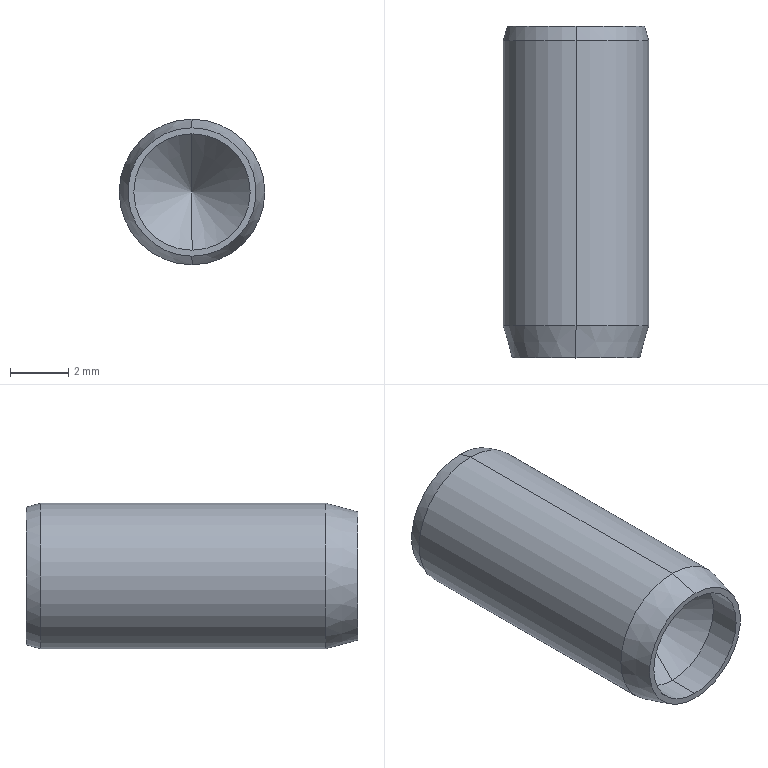Part | STEP file | 1 solid | 25 faces | box 5 x 11.4 x 5 mm | volume 186.144 mm3 | cone 10 | plane 9 | cylinder 6 | commonest cylinder face diameters 1.95 x2 4 x2 5 x2
STEP:
#1=CARTESIAN_POINT('',(0.,7.9,-0.975));
#2=VERTEX_POINT('',#1);
#3=CARTESIAN_POINT('',(0.,8.4,-0.975));
#4=VERTEX_POINT('',#3);
#5=CARTESIAN_POINT('',(0.,11.4,-0.975));
#6=DIRECTION('',(0.,1.,0.));
#7=VECTOR('',#6,1000.);
#8=LINE('',#5,#7);
#9=EDGE_CURVE('',#2,#4,#8,.T.);
#10=ORIENTED_EDGE('',*,*,#9,.F.);
#11=CARTESIAN_POINT('',(0.,7.9,0.975));
#12=VERTEX_POINT('',#11);
#13=CARTESIAN_POINT('',(0.,7.9,0.));
#14=DIRECTION('',(0.,1.,0.));
#15=DIRECTION('',(0.,0.,1.));
#16=AXIS2_PLACEMENT_3D('',#13,#14,#15);
#17=CIRCLE('',#16,0.975);
#18=EDGE_CURVE('',#12,#2,#17,.T.);
#19=ORIENTED_EDGE('',*,*,#18,.F.);
#20=CARTESIAN_POINT('',(0.,8.4,0.975));
#21=VERTEX_POINT('',#20);
#22=CARTESIAN_POINT('',(0.,11.4,0.975));
#23=DIRECTION('',(0.,1.,0.));
#24=VECTOR('',#23,1000.);
#25=LINE('',#22,#24);
#26=EDGE_CURVE('',#12,#21,#25,.T.);
#27=ORIENTED_EDGE('',*,*,#26,.T.);
#28=CARTESIAN_POINT('',(0.,8.4,0.));
#29=DIRECTION('',(0.,-1.,0.));
#30=DIRECTION('',(0.,0.,1.));
#31=AXIS2_PLACEMENT_3D('',#28,#29,#30);
#32=CIRCLE('',#31,0.975);
#33=EDGE_CURVE('',#4,#21,#32,.T.);
#34=ORIENTED_EDGE('',*,*,#33,.F.);
#35=EDGE_LOOP('',(#10,#19,#27,#34));
#36=FACE_OUTER_BOUND('',#35,.T.);
#37=CARTESIAN_POINT('',(0.,11.4,0.));
#38=DIRECTION('',(0.,1.,0.));
#39=DIRECTION('',(0.,0.,1.));
#40=AXIS2_PLACEMENT_3D('',#37,#38,#39);
#41=CYLINDRICAL_SURFACE('',#40,0.975);
#42=ADVANCED_FACE('',(#36),#41,.F.);
#43=CARTESIAN_POINT('',(0.,7.314,0.));
#44=VERTEX_POINT('',#43);
#45=CARTESIAN_POINT('',(0.,7.9,-0.975));
#46=DIRECTION('',(0.,0.515,-0.8572));
#47=VECTOR('',#46,1000.);
#48=LINE('',#45,#47);
#49=EDGE_CURVE('',#44,#2,#48,.T.);
#50=ORIENTED_EDGE('',*,*,#49,.F.);
#51=CARTESIAN_POINT('',(0.,7.9,0.975));
#52=DIRECTION('',(0.,0.515,0.8572));
#53=VECTOR('',#52,1000.);
#54=LINE('',#51,#53);
#55=EDGE_CURVE('',#44,#12,#54,.T.);
#56=ORIENTED_EDGE('',*,*,#55,.T.);
#57=ORIENTED_EDGE('',*,*,#18,.T.);
#58=EDGE_LOOP('',(#50,#56,#57));
#59=FACE_OUTER_BOUND('',#58,.T.);
#60=CARTESIAN_POINT('',(0.,7.9,0.));
#61=DIRECTION('',(0.,1.,0.));
#62=DIRECTION('',(0.,0.,1.));
#63=AXIS2_PLACEMENT_3D('',#60,#61,#62);
#64=CONICAL_SURFACE('',#63,0.975,1.03);
#65=ADVANCED_FACE('',(#59),#64,.F.);
#66=CARTESIAN_POINT('',(1.155,11.38,0.));
#67=VERTEX_POINT('',#66);
#68=CARTESIAN_POINT('',(0.5774,11.38,-1.));
#69=VERTEX_POINT('',#68);
#70=CARTESIAN_POINT('',(1.155,11.38,0.));
#71=CARTESIAN_POINT('',(1.104,11.329,-0.08728));
#72=CARTESIAN_POINT('',(1.031,11.272,-0.215));
#73=CARTESIAN_POINT('',(0.9596,11.243,-0.338));
#74=CARTESIAN_POINT('',(0.9129,11.229,-0.4189));
#75=CARTESIAN_POINT('',(0.889,11.226,-0.4602));
#76=CARTESIAN_POINT('',(0.7793,11.223,-0.6502));
#77=CARTESIAN_POINT('',(0.6828,11.274,-0.8174));
#78=CARTESIAN_POINT('',(0.5774,11.38,-1.));
#79=B_SPLINE_CURVE_WITH_KNOTS('',3,(#70,#71,#72,#73,#74,#75,#76,#77,#78),.UNSPECIFIED.,.F.,.F.,(4,1,2,2,4),(0.,0.25,0.375,0.5,1.),.UNSPECIFIED.);
#80=EDGE_CURVE('',#67,#69,#79,.T.);
#81=ORIENTED_EDGE('',*,*,#80,.T.);
#82=CARTESIAN_POINT('',(0.5774,8.4,-1.));
#83=VERTEX_POINT('',#82);
#84=CARTESIAN_POINT('',(0.5774,8.4,-1.));
#85=DIRECTION('',(0.,1.,0.));
#86=VECTOR('',#85,1000.);
#87=LINE('',#84,#86);
#88=EDGE_CURVE('',#83,#69,#87,.T.);
#89=ORIENTED_EDGE('',*,*,#88,.F.);
#90=CARTESIAN_POINT('',(1.155,8.4,0.));
#91=VERTEX_POINT('',#90);
#92=CARTESIAN_POINT('',(1.155,8.4,0.));
#93=DIRECTION('',(-0.5,0.,-0.866));
#94=VECTOR('',#93,1000.);
#95=LINE('',#92,#94);
#96=EDGE_CURVE('',#91,#83,#95,.T.);
#97=ORIENTED_EDGE('',*,*,#96,.F.);
#98=CARTESIAN_POINT('',(1.155,8.4,0.));
#99=DIRECTION('',(0.,1.,0.));
#100=VECTOR('',#99,1000.);
#101=LINE('',#98,#100);
#102=EDGE_CURVE('',#91,#67,#101,.T.);
#103=ORIENTED_EDGE('',*,*,#102,.T.);
#104=EDGE_LOOP('',(#81,#89,#97,#103));
#105=FACE_OUTER_BOUND('',#104,.T.);
#106=CARTESIAN_POINT('',(1.155,8.4,0.));
#107=DIRECTION('',(0.866,0.,-0.5));
#108=DIRECTION('',(0.,-1.,0.));
#109=AXIS2_PLACEMENT_3D('',#106,#107,#108);
#110=PLANE('',#109);
#111=ADVANCED_FACE('',(#105),#110,.F.);
#112=CARTESIAN_POINT('',(0.,11.225,-1.));
#113=VERTEX_POINT('',#112);
#114=CARTESIAN_POINT('',(0.5774,11.38,-1.));
#115=CARTESIAN_POINT('',(0.3711,11.277,-1.));
#116=CARTESIAN_POINT('',(0.1786,11.225,-1.));
#117=CARTESIAN_POINT('',(0.,11.225,-1.));
#118=B_SPLINE_CURVE_WITH_KNOTS('',3,(#114,#115,#116,#117),.UNSPECIFIED.,.F.,.F.,(4,4),(0.,1.),.UNSPECIFIED.);
#119=EDGE_CURVE('',#69,#113,#118,.T.);
#120=ORIENTED_EDGE('',*,*,#119,.T.);
#121=CARTESIAN_POINT('',(-0.5774,11.38,-1.));
#122=VERTEX_POINT('',#121);
#123=CARTESIAN_POINT('',(0.,11.225,-1.));
#124=CARTESIAN_POINT('',(-0.1786,11.225,-1.));
#125=CARTESIAN_POINT('',(-0.3711,11.277,-1.));
#126=CARTESIAN_POINT('',(-0.5774,11.38,-1.));
#127=B_SPLINE_CURVE_WITH_KNOTS('',3,(#123,#124,#125,#126),.UNSPECIFIED.,.F.,.F.,(4,4),(0.,1.),.UNSPECIFIED.);
#128=EDGE_CURVE('',#113,#122,#127,.T.);
#129=ORIENTED_EDGE('',*,*,#128,.T.);
#130=CARTESIAN_POINT('',(-0.5774,8.4,-1.));
#131=VERTEX_POINT('',#130);
#132=CARTESIAN_POINT('',(-0.5774,8.4,-1.));
#133=DIRECTION('',(0.,1.,0.));
#134=VECTOR('',#133,1000.);
#135=LINE('',#132,#134);
#136=EDGE_CURVE('',#131,#122,#135,.T.);
#137=ORIENTED_EDGE('',*,*,#136,.F.);
#138=CARTESIAN_POINT('',(0.5774,8.4,-1.));
#139=DIRECTION('',(-1.,0.,0.));
#140=VECTOR('',#139,1000.);
#141=LINE('',#138,#140);
#142=EDGE_CURVE('',#83,#131,#141,.T.);
#143=ORIENTED_EDGE('',*,*,#142,.F.);
#144=ORIENTED_EDGE('',*,*,#88,.T.);
#145=EDGE_LOOP('',(#120,#129,#137,#143,#144));
#146=FACE_OUTER_BOUND('',#145,.T.);
#147=CARTESIAN_POINT('',(0.5774,8.4,-1.));
#148=DIRECTION('',(0.,0.,-1.));
#149=DIRECTION('',(0.,-1.,0.));
#150=AXIS2_PLACEMENT_3D('',#147,#148,#149);
#151=PLANE('',#150);
#152=ADVANCED_FACE('',(#146),#151,.F.);
#153=CARTESIAN_POINT('',(-1.155,11.38,0.));
#154=VERTEX_POINT('',#153);
#155=CARTESIAN_POINT('',(-0.5774,11.38,-1.));
#156=CARTESIAN_POINT('',(-0.6277,11.329,-0.9127));
#157=CARTESIAN_POINT('',(-0.7015,11.272,-0.785));
#158=CARTESIAN_POINT('',(-0.7725,11.243,-0.662));
#159=CARTESIAN_POINT('',(-0.8192,11.229,-0.5811));
#160=CARTESIAN_POINT('',(-0.843,11.226,-0.5398));
#161=CARTESIAN_POINT('',(-0.9527,11.223,-0.3498));
#162=CARTESIAN_POINT('',(-1.049,11.274,-0.1826));
#163=CARTESIAN_POINT('',(-1.155,11.38,0.));
#164=B_SPLINE_CURVE_WITH_KNOTS('',3,(#155,#156,#157,#158,#159,#160,#161,#162,#163),.UNSPECIFIED.,.F.,.F.,(4,1,2,2,4),(0.,0.25,0.375,0.5,1.),.UNSPECIFIED.);
#165=EDGE_CURVE('',#122,#154,#164,.T.);
#166=ORIENTED_EDGE('',*,*,#165,.T.);
#167=CARTESIAN_POINT('',(-1.155,8.4,0.));
#168=VERTEX_POINT('',#167);
#169=CARTESIAN_POINT('',(-1.155,8.4,0.));
#170=DIRECTION('',(0.,1.,0.));
#171=VECTOR('',#170,1000.);
#172=LINE('',#169,#171);
#173=EDGE_CURVE('',#168,#154,#172,.T.);
#174=ORIENTED_EDGE('',*,*,#173,.F.);
#175=CARTESIAN_POINT('',(-0.5774,8.4,-1.));
#176=DIRECTION('',(-0.5,0.,0.866));
#177=VECTOR('',#176,1000.);
#178=LINE('',#175,#177);
#179=EDGE_CURVE('',#131,#168,#178,.T.);
#180=ORIENTED_EDGE('',*,*,#179,.F.);
#181=ORIENTED_EDGE('',*,*,#136,.T.);
#182=EDGE_LOOP('',(#166,#174,#180,#181));
#183=FACE_OUTER_BOUND('',#182,.T.);
#184=CARTESIAN_POINT('',(-0.5774,8.4,-1.));
#185=DIRECTION('',(-0.866,0.,-0.5));
#186=DIRECTION('',(-0.5,0.,0.866));
#187=AXIS2_PLACEMENT_3D('',#184,#185,#186);
#188=PLANE('',#187);
#189=ADVANCED_FACE('',(#183),#188,.F.);
#190=CARTESIAN_POINT('',(-0.5774,11.38,1.));
#191=VERTEX_POINT('',#190);
#192=CARTESIAN_POINT('',(-1.155,11.38,0.));
#193=CARTESIAN_POINT('',(-1.104,11.329,0.08728));
#194=CARTESIAN_POINT('',(-1.031,11.272,0.215));
#195=CARTESIAN_POINT('',(-0.9596,11.243,0.338));
#196=CARTESIAN_POINT('',(-0.9129,11.229,0.4189));
#197=CARTESIAN_POINT('',(-0.889,11.226,0.4602));
#198=CARTESIAN_POINT('',(-0.7793,11.223,0.6502));
#199=CARTESIAN_POINT('',(-0.6828,11.274,0.8174));
#200=CARTESIAN_POINT('',(-0.5774,11.38,1.));
#201=B_SPLINE_CURVE_WITH_KNOTS('',3,(#192,#193,#194,#195,#196,#197,#198,#199,#200),.UNSPECIFIED.,.F.,.F.,(4,1,2,2,4),(0.,0.25,0.375,0.5,1.),.UNSPECIFIED.);
#202=EDGE_CURVE('',#154,#191,#201,.T.);
#203=ORIENTED_EDGE('',*,*,#202,.T.);
#204=CARTESIAN_POINT('',(-0.5774,8.4,1.));
#205=VERTEX_POINT('',#204);
#206=CARTESIAN_POINT('',(-0.5774,8.4,1.));
#207=DIRECTION('',(0.,1.,0.));
#208=VECTOR('',#207,1000.);
#209=LINE('',#206,#208);
#210=EDGE_CURVE('',#205,#191,#209,.T.);
#211=ORIENTED_EDGE('',*,*,#210,.F.);
#212=CARTESIAN_POINT('',(-1.155,8.4,0.));
#213=DIRECTION('',(0.5,0.,0.866));
#214=VECTOR('',#213,1000.);
#215=LINE('',#212,#214);
#216=EDGE_CURVE('',#168,#205,#215,.T.);
#217=ORIENTED_EDGE('',*,*,#216,.F.);
#218=ORIENTED_EDGE('',*,*,#173,.T.);
#219=EDGE_LOOP('',(#203,#211,#217,#218));
#220=FACE_OUTER_BOUND('',#219,.T.);
#221=CARTESIAN_POINT('',(-1.155,8.4,0.));
#222=DIRECTION('',(-0.866,0.,0.5));
#223=DIRECTION('',(0.,1.,0.));
#224=AXIS2_PLACEMENT_3D('',#221,#222,#223);
#225=PLANE('',#224);
#226=ADVANCED_FACE('',(#220),#225,.F.);
#227=CARTESIAN_POINT('',(0.,11.225,1.));
#228=VERTEX_POINT('',#227);
#229=CARTESIAN_POINT('',(-0.5774,11.38,1.));
#230=CARTESIAN_POINT('',(-0.3711,11.277,1.));
#231=CARTESIAN_POINT('',(-0.1786,11.225,1.));
#232=CARTESIAN_POINT('',(0.,11.225,1.));
#233=B_SPLINE_CURVE_WITH_KNOTS('',3,(#229,#230,#231,#232),.UNSPECIFIED.,.F.,.F.,(4,4),(0.,1.),.UNSPECIFIED.);
#234=EDGE_CURVE('',#191,#228,#233,.T.);
#235=ORIENTED_EDGE('',*,*,#234,.T.);
#236=CARTESIAN_POINT('',(0.5774,11.38,1.));
#237=VERTEX_POINT('',#236);
#238=CARTESIAN_POINT('',(0.,11.225,1.));
#239=CARTESIAN_POINT('',(0.1786,11.225,1.));
#240=CARTESIAN_POINT('',(0.3711,11.277,1.));
#241=CARTESIAN_POINT('',(0.5774,11.38,1.));
#242=B_SPLINE_CURVE_WITH_KNOTS('',3,(#238,#239,#240,#241),.UNSPECIFIED.,.F.,.F.,(4,4),(0.,1.),.UNSPECIFIED.);
#243=EDGE_CURVE('',#228,#237,#242,.T.);
#244=ORIENTED_EDGE('',*,*,#243,.T.);
#245=CARTESIAN_POINT('',(0.5774,8.4,1.));
#246=VERTEX_POINT('',#245);
#247=CARTESIAN_POINT('',(0.5774,8.4,1.));
#248=DIRECTION('',(0.,1.,0.));
#249=VECTOR('',#248,1000.);
#250=LINE('',#247,#249);
#251=EDGE_CURVE('',#246,#237,#250,.T.);
#252=ORIENTED_EDGE('',*,*,#251,.F.);
#253=CARTESIAN_POINT('',(-0.5774,8.4,1.));
#254=DIRECTION('',(1.,0.,0.));
#255=VECTOR('',#254,1000.);
#256=LINE('',#253,#255);
#257=EDGE_CURVE('',#205,#246,#256,.T.);
#258=ORIENTED_EDGE('',*,*,#257,.F.);
#259=ORIENTED_EDGE('',*,*,#210,.T.);
#260=EDGE_LOOP('',(#235,#244,#252,#258,#259));
#261=FACE_OUTER_BOUND('',#260,.T.);
#262=CARTESIAN_POINT('',(-0.5774,8.4,1.));
#263=DIRECTION('',(0.,0.,1.));
#264=DIRECTION('',(0.,-1.,0.));
#265=AXIS2_PLACEMENT_3D('',#262,#263,#264);
#266=PLANE('',#265);
#267=ADVANCED_FACE('',(#261),#266,.F.);
#268=CARTESIAN_POINT('',(0.5774,11.38,1.));
#269=CARTESIAN_POINT('',(0.6277,11.329,0.9127));
#270=CARTESIAN_POINT('',(0.7015,11.272,0.785));
#271=CARTESIAN_POINT('',(0.7725,11.243,0.662));
#272=CARTESIAN_POINT('',(0.8192,11.229,0.5811));
#273=CARTESIAN_POINT('',(0.843,11.226,0.5398));
#274=CARTESIAN_POINT('',(0.9527,11.223,0.3498));
#275=CARTESIAN_POINT('',(1.049,11.274,0.1826));
#276=CARTESIAN_POINT('',(1.155,11.38,0.));
#277=B_SPLINE_CURVE_WITH_KNOTS('',3,(#268,#269,#270,#271,#272,#273,#274,#275,#276),.UNSPECIFIED.,.F.,.F.,(4,1,2,2,4),(0.,0.25,0.375,0.5,1.),.UNSPECIFIED.);
#278=EDGE_CURVE('',#237,#67,#277,.T.);
#279=ORIENTED_EDGE('',*,*,#278,.T.);
#280=ORIENTED_EDGE('',*,*,#102,.F.);
#281=CARTESIAN_POINT('',(0.5774,8.4,1.));
#282=DIRECTION('',(0.5,0.,-0.866));
#283=VECTOR('',#282,1000.);
#284=LINE('',#281,#283);
#285=EDGE_CURVE('',#246,#91,#284,.T.);
#286=ORIENTED_EDGE('',*,*,#285,.F.);
#287=ORIENTED_EDGE('',*,*,#251,.T.);
#288=EDGE_LOOP('',(#279,#280,#286,#287));
#289=FACE_OUTER_BOUND('',#288,.T.);
#290=CARTESIAN_POINT('',(0.5774,8.4,1.));
#291=DIRECTION('',(0.866,0.,0.5));
#292=DIRECTION('',(0.,-1.,0.));
#293=AXIS2_PLACEMENT_3D('',#290,#291,#292);
#294=PLANE('',#293);
#295=ADVANCED_FACE('',(#289),#294,.F.);
#296=CARTESIAN_POINT('',(0.,8.4,0.));
#297=DIRECTION('',(0.,-1.,0.));
#298=DIRECTION('',(0.,0.,1.));
#299=AXIS2_PLACEMENT_3D('',#296,#297,#298);
#300=CIRCLE('',#299,0.975);
#301=EDGE_CURVE('',#21,#4,#300,.T.);
#302=ORIENTED_EDGE('',*,*,#301,.T.);
#303=ORIENTED_EDGE('',*,*,#33,.T.);
#304=EDGE_LOOP('',(#302,#303));
#305=FACE_BOUND('',#304,.T.);
#306=ORIENTED_EDGE('',*,*,#285,.T.);
#307=ORIENTED_EDGE('',*,*,#96,.T.);
#308=ORIENTED_EDGE('',*,*,#142,.T.);
#309=ORIENTED_EDGE('',*,*,#179,.T.);
#310=ORIENTED_EDGE('',*,*,#216,.T.);
#311=ORIENTED_EDGE('',*,*,#257,.T.);
#312=EDGE_LOOP('',(#306,#307,#308,#309,#310,#311));
#313=FACE_OUTER_BOUND('',#312,.T.);
#314=CARTESIAN_POINT('',(0.,8.4,0.));
#315=DIRECTION('',(0.,1.,0.));
#316=DIRECTION('',(1.,0.,0.));
#317=AXIS2_PLACEMENT_3D('',#314,#315,#316);
#318=PLANE('',#317);
#319=ADVANCED_FACE('',(#305,#313),#318,.T.);
#320=CARTESIAN_POINT('',(0.,11.4,-1.175));
#321=VERTEX_POINT('',#320);
#322=CARTESIAN_POINT('',(0.,11.2,-0.975));
#323=DIRECTION('',(0.,0.7071,-0.7071));
#324=VECTOR('',#323,1000.);
#325=LINE('',#322,#324);
#326=EDGE_CURVE('',#113,#321,#325,.T.);
#327=ORIENTED_EDGE('',*,*,#326,.F.);
#328=ORIENTED_EDGE('',*,*,#119,.F.);
#329=ORIENTED_EDGE('',*,*,#80,.F.);
#330=ORIENTED_EDGE('',*,*,#278,.F.);
#331=ORIENTED_EDGE('',*,*,#243,.F.);
#332=CARTESIAN_POINT('',(0.,11.4,1.175));
#333=VERTEX_POINT('',#332);
#334=CARTESIAN_POINT('',(0.,11.2,0.975));
#335=DIRECTION('',(0.,0.7071,0.7071));
#336=VECTOR('',#335,1000.);
#337=LINE('',#334,#336);
#338=EDGE_CURVE('',#228,#333,#337,.T.);
#339=ORIENTED_EDGE('',*,*,#338,.T.);
#340=CARTESIAN_POINT('',(0.,11.4,0.));
#341=DIRECTION('',(0.,-1.,0.));
#342=DIRECTION('',(0.,0.,1.));
#343=AXIS2_PLACEMENT_3D('',#340,#341,#342);
#344=CIRCLE('',#343,1.175);
#345=EDGE_CURVE('',#321,#333,#344,.T.);
#346=ORIENTED_EDGE('',*,*,#345,.F.);
#347=EDGE_LOOP('',(#327,#328,#329,#330,#331,#339,#346));
#348=FACE_OUTER_BOUND('',#347,.T.);
#349=CARTESIAN_POINT('',(0.,11.2,0.));
#350=DIRECTION('',(0.,1.,0.));
#351=DIRECTION('',(0.,0.,1.));
#352=AXIS2_PLACEMENT_3D('',#349,#350,#351);
#353=CONICAL_SURFACE('',#352,0.975,0.7854);
#354=ADVANCED_FACE('',(#348),#353,.F.);
#355=CARTESIAN_POINT('',(0.,3.1,0.));
#356=VERTEX_POINT('',#355);
#357=CARTESIAN_POINT('',(0.,1.1,2.));
#358=VERTEX_POINT('',#357);
#359=CARTESIAN_POINT('',(0.,3.1,0.));
#360=DIRECTION('',(0.,-0.7071,0.7071));
#361=VECTOR('',#360,1000.);
#362=LINE('',#359,#361);
#363=EDGE_CURVE('',#356,#358,#362,.T.);
#364=ORIENTED_EDGE('',*,*,#363,.F.);
#365=CARTESIAN_POINT('',(0.,1.1,-2.));
#366=VERTEX_POINT('',#365);
#367=CARTESIAN_POINT('',(0.,3.1,0.));
#368=DIRECTION('',(0.,-0.7071,-0.7071));
#369=VECTOR('',#368,1000.);
#370=LINE('',#367,#369);
#371=EDGE_CURVE('',#356,#366,#370,.T.);
#372=ORIENTED_EDGE('',*,*,#371,.T.);
#373=CARTESIAN_POINT('',(0.,1.1,0.));
#374=DIRECTION('',(0.,-1.,0.));
#375=DIRECTION('',(0.,0.,-1.));
#376=AXIS2_PLACEMENT_3D('',#373,#374,#375);
#377=CIRCLE('',#376,2.);
#378=EDGE_CURVE('',#366,#358,#377,.T.);
#379=ORIENTED_EDGE('',*,*,#378,.T.);
#380=EDGE_LOOP('',(#364,#372,#379));
#381=FACE_OUTER_BOUND('',#380,.T.);
#382=CARTESIAN_POINT('',(0.,-996.9,0.));
#383=DIRECTION('',(0.,-1.,0.));
#384=DIRECTION('',(0.,0.,-1.));
#385=AXIS2_PLACEMENT_3D('',#382,#383,#384);
#386=CONICAL_SURFACE('',#385,1000.,0.7854);
#387=ADVANCED_FACE('',(#381),#386,.F.);
#388=CARTESIAN_POINT('',(0.,0.,2.));
#389=VERTEX_POINT('',#388);
#390=CARTESIAN_POINT('',(0.,0.,2.));
#391=DIRECTION('',(0.,-1.,0.));
#392=VECTOR('',#391,1000.);
#393=LINE('',#390,#392);
#394=EDGE_CURVE('',#358,#389,#393,.T.);
#395=ORIENTED_EDGE('',*,*,#394,.F.);
#396=ORIENTED_EDGE('',*,*,#378,.F.);
#397=CARTESIAN_POINT('',(0.,0.,-2.));
#398=VERTEX_POINT('',#397);
#399=CARTESIAN_POINT('',(0.,0.,-2.));
#400=DIRECTION('',(0.,-1.,0.));
#401=VECTOR('',#400,1000.);
#402=LINE('',#399,#401);
#403=EDGE_CURVE('',#366,#398,#402,.T.);
#404=ORIENTED_EDGE('',*,*,#403,.T.);
#405=CARTESIAN_POINT('',(0.,0.,0.));
#406=DIRECTION('',(0.,-1.,0.));
#407=DIRECTION('',(0.,0.,-1.));
#408=AXIS2_PLACEMENT_3D('',#405,#406,#407);
#409=CIRCLE('',#408,2.);
#410=EDGE_CURVE('',#398,#389,#409,.T.);
#411=ORIENTED_EDGE('',*,*,#410,.T.);
#412=EDGE_LOOP('',(#395,#396,#404,#411));
#413=FACE_OUTER_BOUND('',#412,.T.);
#414=CARTESIAN_POINT('',(0.,0.,0.));
#415=DIRECTION('',(0.,-1.,0.));
#416=DIRECTION('',(0.,0.,-1.));
#417=AXIS2_PLACEMENT_3D('',#414,#415,#416);
#418=CYLINDRICAL_SURFACE('',#417,2.);
#419=ADVANCED_FACE('',(#413),#418,.F.);
#420=CARTESIAN_POINT('',(0.,0.,-2.205));
#421=VERTEX_POINT('',#420);
#422=CARTESIAN_POINT('',(0.,1.1,-2.5));
#423=VERTEX_POINT('',#422);
#424=CARTESIAN_POINT('',(0.,1.1,-2.5));
#425=DIRECTION('',(0.,0.9659,-0.2588));
#426=VECTOR('',#425,1000.);
#427=LINE('',#424,#426);
#428=EDGE_CURVE('',#421,#423,#427,.T.);
#429=ORIENTED_EDGE('',*,*,#428,.F.);
#430=CARTESIAN_POINT('',(0.,0.,2.205));
#431=VERTEX_POINT('',#430);
#432=CARTESIAN_POINT('',(0.,0.,0.));
#433=DIRECTION('',(0.,-1.,0.));
#434=DIRECTION('',(0.,0.,1.));
#435=AXIS2_PLACEMENT_3D('',#432,#433,#434);
#436=CIRCLE('',#435,2.205);
#437=EDGE_CURVE('',#431,#421,#436,.T.);
#438=ORIENTED_EDGE('',*,*,#437,.F.);
#439=CARTESIAN_POINT('',(0.,1.1,2.5));
#440=VERTEX_POINT('',#439);
#441=CARTESIAN_POINT('',(0.,1.1,2.5));
#442=DIRECTION('',(0.,0.9659,0.2588));
#443=VECTOR('',#442,1000.);
#444=LINE('',#441,#443);
#445=EDGE_CURVE('',#431,#440,#444,.T.);
#446=ORIENTED_EDGE('',*,*,#445,.T.);
#447=CARTESIAN_POINT('',(0.,1.1,0.));
#448=DIRECTION('',(0.,1.,0.));
#449=DIRECTION('',(0.,0.,1.));
#450=AXIS2_PLACEMENT_3D('',#447,#448,#449);
#451=CIRCLE('',#450,2.5);
#452=EDGE_CURVE('',#423,#440,#451,.T.);
#453=ORIENTED_EDGE('',*,*,#452,.F.);
#454=EDGE_LOOP('',(#429,#438,#446,#453));
#455=FACE_OUTER_BOUND('',#454,.T.);
#456=CARTESIAN_POINT('',(0.,1.1,0.));
#457=DIRECTION('',(0.,1.,0.));
#458=DIRECTION('',(0.,0.,1.));
#459=AXIS2_PLACEMENT_3D('',#456,#457,#458);
#460=CONICAL_SURFACE('',#459,2.5,0.2618);
#461=ADVANCED_FACE('',(#455),#460,.T.);
#462=CARTESIAN_POINT('',(0.,11.4,2.366));
#463=VERTEX_POINT('',#462);
#464=CARTESIAN_POINT('',(0.,10.9,2.5));
#465=VERTEX_POINT('',#464);
#466=CARTESIAN_POINT('',(0.,11.4,2.366));
#467=DIRECTION('',(0.,-0.9659,0.2588));
#468=VECTOR('',#467,1000.);
#469=LINE('',#466,#468);
#470=EDGE_CURVE('',#463,#465,#469,.T.);
#471=ORIENTED_EDGE('',*,*,#470,.F.);
#472=CARTESIAN_POINT('',(0.,11.4,-2.366));
#473=VERTEX_POINT('',#472);
#474=CARTESIAN_POINT('',(0.,11.4,0.));
#475=DIRECTION('',(0.,1.,0.));
#476=DIRECTION('',(0.,0.,1.));
#477=AXIS2_PLACEMENT_3D('',#474,#475,#476);
#478=CIRCLE('',#477,2.366);
#479=EDGE_CURVE('',#473,#463,#478,.T.);
#480=ORIENTED_EDGE('',*,*,#479,.F.);
#481=CARTESIAN_POINT('',(0.,10.9,-2.5));
#482=VERTEX_POINT('',#481);
#483=CARTESIAN_POINT('',(0.,11.4,-2.366));
#484=DIRECTION('',(0.,-0.9659,-0.2588));
#485=VECTOR('',#484,1000.);
#486=LINE('',#483,#485);
#487=EDGE_CURVE('',#473,#482,#486,.T.);
#488=ORIENTED_EDGE('',*,*,#487,.T.);
#489=CARTESIAN_POINT('',(0.,10.9,0.));
#490=DIRECTION('',(0.,-1.,0.));
#491=DIRECTION('',(0.,0.,1.));
#492=AXIS2_PLACEMENT_3D('',#489,#490,#491);
#493=CIRCLE('',#492,2.5);
#494=EDGE_CURVE('',#465,#482,#493,.T.);
#495=ORIENTED_EDGE('',*,*,#494,.F.);
#496=EDGE_LOOP('',(#471,#480,#488,#495));
#497=FACE_OUTER_BOUND('',#496,.T.);
#498=CARTESIAN_POINT('',(0.,11.4,0.));
#499=DIRECTION('',(0.,-1.,0.));
#500=DIRECTION('',(0.,0.,-1.));
#501=AXIS2_PLACEMENT_3D('',#498,#499,#500);
#502=CONICAL_SURFACE('',#501,2.366,0.2618);
#503=ADVANCED_FACE('',(#497),#502,.T.);
#504=ORIENTED_EDGE('',*,*,#410,.F.);
#505=CARTESIAN_POINT('',(0.,0.,0.));
#506=DIRECTION('',(0.,-1.,0.));
#507=DIRECTION('',(0.,0.,-1.));
#508=AXIS2_PLACEMENT_3D('',#505,#506,#507);
#509=CIRCLE('',#508,2.);
#510=EDGE_CURVE('',#389,#398,#509,.T.);
#511=ORIENTED_EDGE('',*,*,#510,.F.);
#512=EDGE_LOOP('',(#504,#511));
#513=FACE_BOUND('',#512,.T.);
#514=ORIENTED_EDGE('',*,*,#437,.T.);
#515=CARTESIAN_POINT('',(0.,0.,0.));
#516=DIRECTION('',(0.,-1.,0.));
#517=DIRECTION('',(0.,0.,1.));
#518=AXIS2_PLACEMENT_3D('',#515,#516,#517);
#519=CIRCLE('',#518,2.205);
#520=EDGE_CURVE('',#421,#431,#519,.T.);
#521=ORIENTED_EDGE('',*,*,#520,.T.);
#522=EDGE_LOOP('',(#514,#521));
#523=FACE_OUTER_BOUND('',#522,.T.);
#524=CARTESIAN_POINT('',(0.,0.,0.));
#525=DIRECTION('',(0.,1.,0.));
#526=DIRECTION('',(1.,0.,0.));
#527=AXIS2_PLACEMENT_3D('',#524,#525,#526);
#528=PLANE('',#527);
#529=ADVANCED_FACE('',(#513,#523),#528,.F.);
#530=CARTESIAN_POINT('',(0.,11.4,0.));
#531=DIRECTION('',(0.,-1.,0.));
#532=DIRECTION('',(0.,0.,1.));
#533=AXIS2_PLACEMENT_3D('',#530,#531,#532);
#534=CIRCLE('',#533,1.175);
#535=EDGE_CURVE('',#333,#321,#534,.T.);
#536=ORIENTED_EDGE('',*,*,#535,.T.);
#537=ORIENTED_EDGE('',*,*,#345,.T.);
#538=EDGE_LOOP('',(#536,#537));
#539=FACE_BOUND('',#538,.T.);
#540=ORIENTED_EDGE('',*,*,#479,.T.);
#541=CARTESIAN_POINT('',(0.,11.4,0.));
#542=DIRECTION('',(0.,1.,0.));
#543=DIRECTION('',(0.,0.,1.));
#544=AXIS2_PLACEMENT_3D('',#541,#542,#543);
#545=CIRCLE('',#544,2.366);
#546=EDGE_CURVE('',#463,#473,#545,.T.);
#547=ORIENTED_EDGE('',*,*,#546,.T.);
#548=EDGE_LOOP('',(#540,#547));
#549=FACE_OUTER_BOUND('',#548,.T.);
#550=CARTESIAN_POINT('',(0.,11.4,0.));
#551=DIRECTION('',(0.,1.,0.));
#552=DIRECTION('',(1.,0.,0.));
#553=AXIS2_PLACEMENT_3D('',#550,#551,#552);
#554=PLANE('',#553);
#555=ADVANCED_FACE('',(#539,#549),#554,.T.);
#556=CARTESIAN_POINT('',(0.,11.4,2.5));
#557=DIRECTION('',(0.,-1.,0.));
#558=VECTOR('',#557,1000.);
#559=LINE('',#556,#558);
#560=EDGE_CURVE('',#465,#440,#559,.T.);
#561=ORIENTED_EDGE('',*,*,#560,.F.);
#562=ORIENTED_EDGE('',*,*,#494,.T.);
#563=CARTESIAN_POINT('',(0.,11.4,-2.5));
#564=DIRECTION('',(0.,-1.,0.));
#565=VECTOR('',#564,1000.);
#566=LINE('',#563,#565);
#567=EDGE_CURVE('',#482,#423,#566,.T.);
#568=ORIENTED_EDGE('',*,*,#567,.T.);
#569=ORIENTED_EDGE('',*,*,#452,.T.);
#570=EDGE_LOOP('',(#561,#562,#568,#569));
#571=FACE_OUTER_BOUND('',#570,.T.);
#572=CARTESIAN_POINT('',(0.,11.4,0.));
#573=DIRECTION('',(0.,-1.,0.));
#574=DIRECTION('',(0.,0.,-1.));
#575=AXIS2_PLACEMENT_3D('',#572,#573,#574);
#576=CYLINDRICAL_SURFACE('',#575,2.5);
#577=ADVANCED_FACE('',(#571),#576,.T.);
#578=CARTESIAN_POINT('',(0.,10.9,0.));
#579=DIRECTION('',(0.,-1.,0.));
#580=DIRECTION('',(0.,0.,1.));
#581=AXIS2_PLACEMENT_3D('',#578,#579,#580);
#582=CIRCLE('',#581,2.5);
#583=EDGE_CURVE('',#482,#465,#582,.T.);
#584=ORIENTED_EDGE('',*,*,#583,.T.);
#585=ORIENTED_EDGE('',*,*,#560,.T.);
#586=CARTESIAN_POINT('',(0.,1.1,0.));
#587=DIRECTION('',(0.,1.,0.));
#588=DIRECTION('',(0.,0.,1.));
#589=AXIS2_PLACEMENT_3D('',#586,#587,#588);
#590=CIRCLE('',#589,2.5);
#591=EDGE_CURVE('',#440,#423,#590,.T.);
#592=ORIENTED_EDGE('',*,*,#591,.T.);
#593=ORIENTED_EDGE('',*,*,#567,.F.);
#594=EDGE_LOOP('',(#584,#585,#592,#593));
#595=FACE_OUTER_BOUND('',#594,.T.);
#596=CARTESIAN_POINT('',(0.,11.4,0.));
#597=DIRECTION('',(0.,-1.,0.));
#598=DIRECTION('',(0.,0.,-1.));
#599=AXIS2_PLACEMENT_3D('',#596,#597,#598);
#600=CYLINDRICAL_SURFACE('',#599,2.5);
#601=ADVANCED_FACE('',(#595),#600,.T.);
#602=ORIENTED_EDGE('',*,*,#546,.F.);
#603=ORIENTED_EDGE('',*,*,#470,.T.);
#604=ORIENTED_EDGE('',*,*,#583,.F.);
#605=ORIENTED_EDGE('',*,*,#487,.F.);
#606=EDGE_LOOP('',(#602,#603,#604,#605));
#607=FACE_OUTER_BOUND('',#606,.T.);
#608=CARTESIAN_POINT('',(0.,11.4,0.));
#609=DIRECTION('',(0.,-1.,0.));
#610=DIRECTION('',(0.,0.,-1.));
#611=AXIS2_PLACEMENT_3D('',#608,#609,#610);
#612=CONICAL_SURFACE('',#611,2.366,0.2618);
#613=ADVANCED_FACE('',(#607),#612,.T.);
#614=ORIENTED_EDGE('',*,*,#520,.F.);
#615=ORIENTED_EDGE('',*,*,#428,.T.);
#616=ORIENTED_EDGE('',*,*,#591,.F.);
#617=ORIENTED_EDGE('',*,*,#445,.F.);
#618=EDGE_LOOP('',(#614,#615,#616,#617));
#619=FACE_OUTER_BOUND('',#618,.T.);
#620=CARTESIAN_POINT('',(0.,1.1,0.));
#621=DIRECTION('',(0.,1.,0.));
#622=DIRECTION('',(0.,0.,1.));
#623=AXIS2_PLACEMENT_3D('',#620,#621,#622);
#624=CONICAL_SURFACE('',#623,2.5,0.2618);
#625=ADVANCED_FACE('',(#619),#624,.T.);
#626=CARTESIAN_POINT('',(0.,1.1,0.));
#627=DIRECTION('',(0.,-1.,0.));
#628=DIRECTION('',(0.,0.,-1.));
#629=AXIS2_PLACEMENT_3D('',#626,#627,#628);
#630=CIRCLE('',#629,2.);
#631=EDGE_CURVE('',#358,#366,#630,.T.);
#632=ORIENTED_EDGE('',*,*,#631,.F.);
#633=ORIENTED_EDGE('',*,*,#394,.T.);
#634=ORIENTED_EDGE('',*,*,#510,.T.);
#635=ORIENTED_EDGE('',*,*,#403,.F.);
#636=EDGE_LOOP('',(#632,#633,#634,#635));
#637=FACE_OUTER_BOUND('',#636,.T.);
#638=CARTESIAN_POINT('',(0.,0.,0.));
#639=DIRECTION('',(0.,-1.,0.));
#640=DIRECTION('',(0.,0.,-1.));
#641=AXIS2_PLACEMENT_3D('',#638,#639,#640);
#642=CYLINDRICAL_SURFACE('',#641,2.);
#643=ADVANCED_FACE('',(#637),#642,.F.);
#644=ORIENTED_EDGE('',*,*,#371,.F.);
#645=ORIENTED_EDGE('',*,*,#363,.T.);
#646=ORIENTED_EDGE('',*,*,#631,.T.);
#647=EDGE_LOOP('',(#644,#645,#646));
#648=FACE_OUTER_BOUND('',#647,.T.);
#649=CARTESIAN_POINT('',(0.,-996.9,0.));
#650=DIRECTION('',(0.,-1.,0.));
#651=DIRECTION('',(0.,0.,-1.));
#652=AXIS2_PLACEMENT_3D('',#649,#650,#651);
#653=CONICAL_SURFACE('',#652,1000.,0.7854);
#654=ADVANCED_FACE('',(#648),#653,.F.);
#655=ORIENTED_EDGE('',*,*,#128,.F.);
#656=ORIENTED_EDGE('',*,*,#326,.T.);
#657=ORIENTED_EDGE('',*,*,#535,.F.);
#658=ORIENTED_EDGE('',*,*,#338,.F.);
#659=ORIENTED_EDGE('',*,*,#234,.F.);
#660=ORIENTED_EDGE('',*,*,#202,.F.);
#661=ORIENTED_EDGE('',*,*,#165,.F.);
#662=EDGE_LOOP('',(#655,#656,#657,#658,#659,#660,#661));
#663=FACE_OUTER_BOUND('',#662,.T.);
#664=CARTESIAN_POINT('',(0.,11.2,0.));
#665=DIRECTION('',(0.,1.,0.));
#666=DIRECTION('',(0.,0.,1.));
#667=AXIS2_PLACEMENT_3D('',#664,#665,#666);
#668=CONICAL_SURFACE('',#667,0.975,0.7854);
#669=ADVANCED_FACE('',(#663),#668,.F.);
#670=ORIENTED_EDGE('',*,*,#55,.F.);
#671=ORIENTED_EDGE('',*,*,#49,.T.);
#672=CARTESIAN_POINT('',(0.,7.9,0.));
#673=DIRECTION('',(0.,1.,0.));
#674=DIRECTION('',(0.,0.,1.));
#675=AXIS2_PLACEMENT_3D('',#672,#673,#674);
#676=CIRCLE('',#675,0.975);
#677=EDGE_CURVE('',#2,#12,#676,.T.);
#678=ORIENTED_EDGE('',*,*,#677,.T.);
#679=EDGE_LOOP('',(#670,#671,#678));
#680=FACE_OUTER_BOUND('',#679,.T.);
#681=CARTESIAN_POINT('',(0.,7.9,0.));
#682=DIRECTION('',(0.,1.,0.));
#683=DIRECTION('',(0.,0.,1.));
#684=AXIS2_PLACEMENT_3D('',#681,#682,#683);
#685=CONICAL_SURFACE('',#684,0.975,1.03);
#686=ADVANCED_FACE('',(#680),#685,.F.);
#687=ORIENTED_EDGE('',*,*,#677,.F.);
#688=ORIENTED_EDGE('',*,*,#9,.T.);
#689=ORIENTED_EDGE('',*,*,#301,.F.);
#690=ORIENTED_EDGE('',*,*,#26,.F.);
#691=EDGE_LOOP('',(#687,#688,#689,#690));
#692=FACE_OUTER_BOUND('',#691,.T.);
#693=CARTESIAN_POINT('',(0.,11.4,0.));
#694=DIRECTION('',(0.,1.,0.));
#695=DIRECTION('',(0.,0.,1.));
#696=AXIS2_PLACEMENT_3D('',#693,#694,#695);
#697=CYLINDRICAL_SURFACE('',#696,0.975);
#698=ADVANCED_FACE('',(#692),#697,.F.);
#699=CLOSED_SHELL('',(#42,#65,#111,#152,#189,#226,#267,#295,#319,#354,#387,#419,#461,#503,#529,#555,#577,#601,#613,#625,#643,#654,#669,#686,#698));
#700=MANIFOLD_SOLID_BREP('',#699);
#701=CARTESIAN_POINT('',(0.,0.,0.));
#702=DIRECTION('',(0.,0.,1.));
#703=DIRECTION('',(1.,0.,0.));
#704=AXIS2_PLACEMENT_3D('',#701,#702,#703);
#705=(LENGTH_UNIT()NAMED_UNIT(*)SI_UNIT(.MILLI.,.METRE.));
#706=UNCERTAINTY_MEASURE_WITH_UNIT(LENGTH_MEASURE(0.00001),#705,'','');
#707=(NAMED_UNIT(*)PLANE_ANGLE_UNIT()SI_UNIT($,.RADIAN.));
#708=(NAMED_UNIT(*)SI_UNIT($,.STERADIAN.)SOLID_ANGLE_UNIT());
#709=(GEOMETRIC_REPRESENTATION_CONTEXT(3)GLOBAL_UNCERTAINTY_ASSIGNED_CONTEXT((#706))GLOBAL_UNIT_ASSIGNED_CONTEXT((#705,#707,#708))REPRESENTATION_CONTEXT('',''));
#710=ADVANCED_BREP_SHAPE_REPRESENTATION('',(#700,#704),#709);